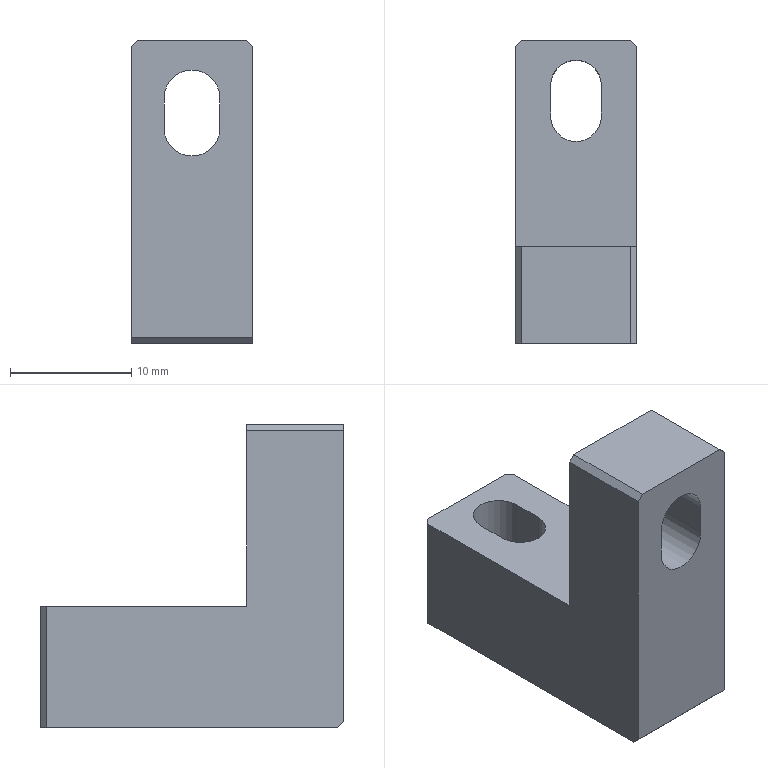Part | SolidWorks | features ICE 3, Chamfer 1, Extrusion 1, MoveFace 1 | 1 solid | 22 faces | box 10 x 25 x 25 mm | volume 3226 mm3 | plane 17 | cylinder 5 | commonest cylinder face diameters 4.6 x3 4.2 x2
STEP:
#1=CARTESIAN_POINT('',(5.,-5.,22.55));
#2=VERTEX_POINT('',#1);
#3=CARTESIAN_POINT('',(7.3,-5.,20.25));
#4=VERTEX_POINT('',#3);
#5=CARTESIAN_POINT('',(5.,-5.,20.25));
#6=DIRECTION('',(0.,1.,0.));
#7=DIRECTION('',(0.,0.,1.));
#8=AXIS2_PLACEMENT_3D('',#5,#6,#7);
#9=CIRCLE('',#8,2.3);
#10=EDGE_CURVE('',#2,#4,#9,.T.);
#11=ORIENTED_EDGE('',*,*,#10,.F.);
#12=CARTESIAN_POINT('',(5.,3.,22.55));
#13=VERTEX_POINT('',#12);
#14=CARTESIAN_POINT('',(5.,-2.,22.55));
#15=DIRECTION('',(0.,1.,0.));
#16=VECTOR('',#15,1000.);
#17=LINE('',#14,#16);
#18=EDGE_CURVE('',#2,#13,#17,.T.);
#19=ORIENTED_EDGE('',*,*,#18,.T.);
#20=CARTESIAN_POINT('',(7.3,3.,20.25));
#21=VERTEX_POINT('',#20);
#22=CARTESIAN_POINT('',(5.,3.,20.25));
#23=DIRECTION('',(0.,1.,0.));
#24=DIRECTION('',(0.,0.,1.));
#25=AXIS2_PLACEMENT_3D('',#22,#23,#24);
#26=CIRCLE('',#25,2.3);
#27=EDGE_CURVE('',#13,#21,#26,.T.);
#28=ORIENTED_EDGE('',*,*,#27,.T.);
#29=CARTESIAN_POINT('',(7.3,-2.,20.25));
#30=DIRECTION('',(0.,1.,0.));
#31=VECTOR('',#30,1000.);
#32=LINE('',#29,#31);
#33=EDGE_CURVE('',#4,#21,#32,.T.);
#34=ORIENTED_EDGE('',*,*,#33,.F.);
#35=EDGE_LOOP('',(#11,#19,#28,#34));
#36=FACE_OUTER_BOUND('',#35,.T.);
#37=CARTESIAN_POINT('',(5.,-2.,20.25));
#38=DIRECTION('',(0.,1.,0.));
#39=DIRECTION('',(0.,0.,1.));
#40=AXIS2_PLACEMENT_3D('',#37,#38,#39);
#41=CYLINDRICAL_SURFACE('',#40,2.3);
#42=ADVANCED_FACE('',(#36),#41,.F.);
#43=CARTESIAN_POINT('',(2.9,16.25,10.));
#44=VERTEX_POINT('',#43);
#45=CARTESIAN_POINT('',(2.9,13.75,10.));
#46=VERTEX_POINT('',#45);
#47=CARTESIAN_POINT('',(2.9,16.25,10.));
#48=DIRECTION('',(0.,-1.,0.));
#49=VECTOR('',#48,1000.);
#50=LINE('',#47,#49);
#51=EDGE_CURVE('',#44,#46,#50,.T.);
#52=ORIENTED_EDGE('',*,*,#51,.F.);
#53=CARTESIAN_POINT('',(7.1,16.25,10.));
#54=VERTEX_POINT('',#53);
#55=CARTESIAN_POINT('',(5.,16.25,10.));
#56=DIRECTION('',(0.,0.,1.));
#57=DIRECTION('',(1.,0.,0.));
#58=AXIS2_PLACEMENT_3D('',#55,#56,#57);
#59=CIRCLE('',#58,2.1);
#60=EDGE_CURVE('',#54,#44,#59,.T.);
#61=ORIENTED_EDGE('',*,*,#60,.F.);
#62=CARTESIAN_POINT('',(7.1,13.75,10.));
#63=VERTEX_POINT('',#62);
#64=CARTESIAN_POINT('',(7.1,16.25,10.));
#65=DIRECTION('',(0.,1.,0.));
#66=VECTOR('',#65,1000.);
#67=LINE('',#64,#66);
#68=EDGE_CURVE('',#63,#54,#67,.T.);
#69=ORIENTED_EDGE('',*,*,#68,.F.);
#70=CARTESIAN_POINT('',(5.,13.75,10.));
#71=DIRECTION('',(0.,0.,1.));
#72=DIRECTION('',(1.,0.,0.));
#73=AXIS2_PLACEMENT_3D('',#70,#71,#72);
#74=CIRCLE('',#73,2.1);
#75=EDGE_CURVE('',#46,#63,#74,.T.);
#76=ORIENTED_EDGE('',*,*,#75,.F.);
#77=EDGE_LOOP('',(#52,#61,#69,#76));
#78=FACE_BOUND('',#77,.T.);
#79=CARTESIAN_POINT('',(10.,3.,10.));
#80=VERTEX_POINT('',#79);
#81=CARTESIAN_POINT('',(10.,19.5,10.));
#82=VERTEX_POINT('',#81);
#83=CARTESIAN_POINT('',(10.,0.,10.));
#84=DIRECTION('',(0.,1.,0.));
#85=VECTOR('',#84,1000.);
#86=LINE('',#83,#85);
#87=EDGE_CURVE('',#80,#82,#86,.T.);
#88=ORIENTED_EDGE('',*,*,#87,.T.);
#89=CARTESIAN_POINT('',(9.5,20.,10.));
#90=VERTEX_POINT('',#89);
#91=CARTESIAN_POINT('',(9.5,20.,10.));
#92=DIRECTION('',(-0.7071,0.7071,0.));
#93=VECTOR('',#92,1000.);
#94=LINE('',#91,#93);
#95=EDGE_CURVE('',#82,#90,#94,.T.);
#96=ORIENTED_EDGE('',*,*,#95,.T.);
#97=CARTESIAN_POINT('',(0.5,20.,10.));
#98=VERTEX_POINT('',#97);
#99=CARTESIAN_POINT('',(0.,20.,10.));
#100=DIRECTION('',(-1.,0.,0.));
#101=VECTOR('',#100,1000.);
#102=LINE('',#99,#101);
#103=EDGE_CURVE('',#90,#98,#102,.T.);
#104=ORIENTED_EDGE('',*,*,#103,.T.);
#105=CARTESIAN_POINT('',(0.,19.5,10.));
#106=VERTEX_POINT('',#105);
#107=CARTESIAN_POINT('',(0.,19.5,10.));
#108=DIRECTION('',(-0.7071,-0.7071,0.));
#109=VECTOR('',#108,1000.);
#110=LINE('',#107,#109);
#111=EDGE_CURVE('',#98,#106,#110,.T.);
#112=ORIENTED_EDGE('',*,*,#111,.T.);
#113=CARTESIAN_POINT('',(0.,3.,10.));
#114=VERTEX_POINT('',#113);
#115=CARTESIAN_POINT('',(0.,0.,10.));
#116=DIRECTION('',(0.,-1.,0.));
#117=VECTOR('',#116,1000.);
#118=LINE('',#115,#117);
#119=EDGE_CURVE('',#106,#114,#118,.T.);
#120=ORIENTED_EDGE('',*,*,#119,.T.);
#121=CARTESIAN_POINT('',(0.,3.,10.));
#122=DIRECTION('',(-1.,0.,0.));
#123=VECTOR('',#122,1000.);
#124=LINE('',#121,#123);
#125=EDGE_CURVE('',#80,#114,#124,.T.);
#126=ORIENTED_EDGE('',*,*,#125,.F.);
#127=EDGE_LOOP('',(#88,#96,#104,#112,#120,#126));
#128=FACE_OUTER_BOUND('',#127,.T.);
#129=CARTESIAN_POINT('',(0.,0.,10.));
#130=DIRECTION('',(0.,0.,-1.));
#131=DIRECTION('',(-1.,0.,0.));
#132=AXIS2_PLACEMENT_3D('',#129,#130,#131);
#133=PLANE('',#132);
#134=ADVANCED_FACE('',(#78,#128),#133,.F.);
#135=CARTESIAN_POINT('',(0.,19.5,0.));
#136=VERTEX_POINT('',#135);
#137=CARTESIAN_POINT('',(0.,-4.5,0.));
#138=VERTEX_POINT('',#137);
#139=CARTESIAN_POINT('',(0.,0.,0.));
#140=DIRECTION('',(0.,-1.,0.));
#141=VECTOR('',#140,1000.);
#142=LINE('',#139,#141);
#143=EDGE_CURVE('',#136,#138,#142,.T.);
#144=ORIENTED_EDGE('',*,*,#143,.T.);
#145=CARTESIAN_POINT('',(0.,-5.,0.5));
#146=VERTEX_POINT('',#145);
#147=CARTESIAN_POINT('',(0.,-5.,0.5));
#148=DIRECTION('',(0.,-0.7071,0.7071));
#149=VECTOR('',#148,1000.);
#150=LINE('',#147,#149);
#151=EDGE_CURVE('',#138,#146,#150,.T.);
#152=ORIENTED_EDGE('',*,*,#151,.T.);
#153=CARTESIAN_POINT('',(0.,-5.,24.5));
#154=VERTEX_POINT('',#153);
#155=CARTESIAN_POINT('',(0.,-5.,10.));
#156=DIRECTION('',(0.,0.,-1.));
#157=VECTOR('',#156,1000.);
#158=LINE('',#155,#157);
#159=EDGE_CURVE('',#154,#146,#158,.T.);
#160=ORIENTED_EDGE('',*,*,#159,.F.);
#161=CARTESIAN_POINT('',(0.,3.,24.5));
#162=VERTEX_POINT('',#161);
#163=CARTESIAN_POINT('',(0.,0.,24.5));
#164=DIRECTION('',(0.,1.,0.));
#165=VECTOR('',#164,1000.);
#166=LINE('',#163,#165);
#167=EDGE_CURVE('',#154,#162,#166,.T.);
#168=ORIENTED_EDGE('',*,*,#167,.T.);
#169=CARTESIAN_POINT('',(0.,3.,25.));
#170=DIRECTION('',(0.,0.,-1.));
#171=VECTOR('',#170,1000.);
#172=LINE('',#169,#171);
#173=EDGE_CURVE('',#162,#114,#172,.T.);
#174=ORIENTED_EDGE('',*,*,#173,.T.);
#175=ORIENTED_EDGE('',*,*,#119,.F.);
#176=CARTESIAN_POINT('',(0.,19.5,10.));
#177=DIRECTION('',(0.,0.,-1.));
#178=VECTOR('',#177,1000.);
#179=LINE('',#176,#178);
#180=EDGE_CURVE('',#106,#136,#179,.T.);
#181=ORIENTED_EDGE('',*,*,#180,.T.);
#182=EDGE_LOOP('',(#144,#152,#160,#168,#174,#175,#181));
#183=FACE_OUTER_BOUND('',#182,.T.);
#184=CARTESIAN_POINT('',(0.,0.,10.));
#185=DIRECTION('',(1.,0.,0.));
#186=DIRECTION('',(0.,1.,0.));
#187=AXIS2_PLACEMENT_3D('',#184,#185,#186);
#188=PLANE('',#187);
#189=ADVANCED_FACE('',(#183),#188,.F.);
#190=CARTESIAN_POINT('',(2.7,-5.,17.75));
#191=VERTEX_POINT('',#190);
#192=CARTESIAN_POINT('',(2.7,-5.,20.25));
#193=VERTEX_POINT('',#192);
#194=CARTESIAN_POINT('',(2.7,-5.,10.));
#195=DIRECTION('',(0.,0.,1.));
#196=VECTOR('',#195,1000.);
#197=LINE('',#194,#196);
#198=EDGE_CURVE('',#191,#193,#197,.T.);
#199=ORIENTED_EDGE('',*,*,#198,.T.);
#200=CARTESIAN_POINT('',(5.,-5.,20.25));
#201=DIRECTION('',(0.,1.,0.));
#202=DIRECTION('',(0.,0.,1.));
#203=AXIS2_PLACEMENT_3D('',#200,#201,#202);
#204=CIRCLE('',#203,2.3);
#205=EDGE_CURVE('',#193,#2,#204,.T.);
#206=ORIENTED_EDGE('',*,*,#205,.T.);
#207=ORIENTED_EDGE('',*,*,#10,.T.);
#208=CARTESIAN_POINT('',(7.3,-5.,17.75));
#209=VERTEX_POINT('',#208);
#210=CARTESIAN_POINT('',(7.3,-5.,10.));
#211=DIRECTION('',(0.,0.,-1.));
#212=VECTOR('',#211,1000.);
#213=LINE('',#210,#212);
#214=EDGE_CURVE('',#4,#209,#213,.T.);
#215=ORIENTED_EDGE('',*,*,#214,.T.);
#216=CARTESIAN_POINT('',(5.,-5.,17.75));
#217=DIRECTION('',(0.,1.,0.));
#218=DIRECTION('',(0.,0.,1.));
#219=AXIS2_PLACEMENT_3D('',#216,#217,#218);
#220=CIRCLE('',#219,2.3);
#221=EDGE_CURVE('',#209,#191,#220,.T.);
#222=ORIENTED_EDGE('',*,*,#221,.T.);
#223=EDGE_LOOP('',(#199,#206,#207,#215,#222));
#224=FACE_BOUND('',#223,.T.);
#225=ORIENTED_EDGE('',*,*,#159,.T.);
#226=CARTESIAN_POINT('',(10.,-5.,0.5));
#227=VERTEX_POINT('',#226);
#228=CARTESIAN_POINT('',(10.,-5.,0.5));
#229=DIRECTION('',(1.,0.,0.));
#230=VECTOR('',#229,1000.);
#231=LINE('',#228,#230);
#232=EDGE_CURVE('',#146,#227,#231,.T.);
#233=ORIENTED_EDGE('',*,*,#232,.T.);
#234=CARTESIAN_POINT('',(10.,-5.,24.5));
#235=VERTEX_POINT('',#234);
#236=CARTESIAN_POINT('',(10.,-5.,10.));
#237=DIRECTION('',(0.,0.,-1.));
#238=VECTOR('',#237,1000.);
#239=LINE('',#236,#238);
#240=EDGE_CURVE('',#235,#227,#239,.T.);
#241=ORIENTED_EDGE('',*,*,#240,.F.);
#242=CARTESIAN_POINT('',(9.5,-5.,25.));
#243=VERTEX_POINT('',#242);
#244=CARTESIAN_POINT('',(9.5,-5.,25.));
#245=DIRECTION('',(-0.7071,0.,0.7071));
#246=VECTOR('',#245,1000.);
#247=LINE('',#244,#246);
#248=EDGE_CURVE('',#235,#243,#247,.T.);
#249=ORIENTED_EDGE('',*,*,#248,.T.);
#250=CARTESIAN_POINT('',(0.5,-5.,25.));
#251=VERTEX_POINT('',#250);
#252=CARTESIAN_POINT('',(0.,-5.,25.));
#253=DIRECTION('',(1.,0.,0.));
#254=VECTOR('',#253,1000.);
#255=LINE('',#252,#254);
#256=EDGE_CURVE('',#251,#243,#255,.T.);
#257=ORIENTED_EDGE('',*,*,#256,.F.);
#258=CARTESIAN_POINT('',(0.5,-5.,25.));
#259=DIRECTION('',(-0.7071,0.,-0.7071));
#260=VECTOR('',#259,1000.);
#261=LINE('',#258,#260);
#262=EDGE_CURVE('',#251,#154,#261,.T.);
#263=ORIENTED_EDGE('',*,*,#262,.T.);
#264=EDGE_LOOP('',(#225,#233,#241,#249,#257,#263));
#265=FACE_OUTER_BOUND('',#264,.T.);
#266=CARTESIAN_POINT('',(0.,-5.,10.));
#267=DIRECTION('',(0.,1.,0.));
#268=DIRECTION('',(0.,0.,1.));
#269=AXIS2_PLACEMENT_3D('',#266,#267,#268);
#270=PLANE('',#269);
#271=ADVANCED_FACE('',(#224,#265),#270,.F.);
#272=ORIENTED_EDGE('',*,*,#240,.T.);
#273=CARTESIAN_POINT('',(10.,-4.5,0.));
#274=VERTEX_POINT('',#273);
#275=CARTESIAN_POINT('',(10.,-5.,0.5));
#276=DIRECTION('',(0.,0.7071,-0.7071));
#277=VECTOR('',#276,1000.);
#278=LINE('',#275,#277);
#279=EDGE_CURVE('',#227,#274,#278,.T.);
#280=ORIENTED_EDGE('',*,*,#279,.T.);
#281=CARTESIAN_POINT('',(10.,19.5,0.));
#282=VERTEX_POINT('',#281);
#283=CARTESIAN_POINT('',(10.,0.,0.));
#284=DIRECTION('',(0.,1.,0.));
#285=VECTOR('',#284,1000.);
#286=LINE('',#283,#285);
#287=EDGE_CURVE('',#274,#282,#286,.T.);
#288=ORIENTED_EDGE('',*,*,#287,.T.);
#289=CARTESIAN_POINT('',(10.,19.5,10.));
#290=DIRECTION('',(0.,0.,1.));
#291=VECTOR('',#290,1000.);
#292=LINE('',#289,#291);
#293=EDGE_CURVE('',#282,#82,#292,.T.);
#294=ORIENTED_EDGE('',*,*,#293,.T.);
#295=ORIENTED_EDGE('',*,*,#87,.F.);
#296=CARTESIAN_POINT('',(10.,3.,24.5));
#297=VERTEX_POINT('',#296);
#298=CARTESIAN_POINT('',(10.,3.,25.));
#299=DIRECTION('',(0.,0.,-1.));
#300=VECTOR('',#299,1000.);
#301=LINE('',#298,#300);
#302=EDGE_CURVE('',#297,#80,#301,.T.);
#303=ORIENTED_EDGE('',*,*,#302,.F.);
#304=CARTESIAN_POINT('',(10.,0.,24.5));
#305=DIRECTION('',(0.,-1.,0.));
#306=VECTOR('',#305,1000.);
#307=LINE('',#304,#306);
#308=EDGE_CURVE('',#297,#235,#307,.T.);
#309=ORIENTED_EDGE('',*,*,#308,.T.);
#310=EDGE_LOOP('',(#272,#280,#288,#294,#295,#303,#309));
#311=FACE_OUTER_BOUND('',#310,.T.);
#312=CARTESIAN_POINT('',(10.,0.,10.));
#313=DIRECTION('',(-1.,0.,0.));
#314=DIRECTION('',(0.,-1.,0.));
#315=AXIS2_PLACEMENT_3D('',#312,#313,#314);
#316=PLANE('',#315);
#317=ADVANCED_FACE('',(#311),#316,.F.);
#318=ORIENTED_EDGE('',*,*,#103,.F.);
#319=CARTESIAN_POINT('',(9.5,20.,0.));
#320=VERTEX_POINT('',#319);
#321=CARTESIAN_POINT('',(9.5,20.,10.));
#322=DIRECTION('',(0.,0.,-1.));
#323=VECTOR('',#322,1000.);
#324=LINE('',#321,#323);
#325=EDGE_CURVE('',#90,#320,#324,.T.);
#326=ORIENTED_EDGE('',*,*,#325,.T.);
#327=CARTESIAN_POINT('',(0.5,20.,0.));
#328=VERTEX_POINT('',#327);
#329=CARTESIAN_POINT('',(0.,20.,0.));
#330=DIRECTION('',(-1.,0.,0.));
#331=VECTOR('',#330,1000.);
#332=LINE('',#329,#331);
#333=EDGE_CURVE('',#320,#328,#332,.T.);
#334=ORIENTED_EDGE('',*,*,#333,.T.);
#335=CARTESIAN_POINT('',(0.5,20.,10.));
#336=DIRECTION('',(0.,0.,1.));
#337=VECTOR('',#336,1000.);
#338=LINE('',#335,#337);
#339=EDGE_CURVE('',#328,#98,#338,.T.);
#340=ORIENTED_EDGE('',*,*,#339,.T.);
#341=EDGE_LOOP('',(#318,#326,#334,#340));
#342=FACE_OUTER_BOUND('',#341,.T.);
#343=CARTESIAN_POINT('',(0.,20.,10.));
#344=DIRECTION('',(0.,-1.,0.));
#345=DIRECTION('',(0.,0.,-1.));
#346=AXIS2_PLACEMENT_3D('',#343,#344,#345);
#347=PLANE('',#346);
#348=ADVANCED_FACE('',(#342),#347,.F.);
#349=CARTESIAN_POINT('',(7.1,16.25,0.));
#350=VERTEX_POINT('',#349);
#351=CARTESIAN_POINT('',(2.9,16.25,0.));
#352=VERTEX_POINT('',#351);
#353=CARTESIAN_POINT('',(5.,16.25,0.));
#354=DIRECTION('',(0.,0.,1.));
#355=DIRECTION('',(1.,0.,0.));
#356=AXIS2_PLACEMENT_3D('',#353,#354,#355);
#357=CIRCLE('',#356,2.1);
#358=EDGE_CURVE('',#350,#352,#357,.T.);
#359=ORIENTED_EDGE('',*,*,#358,.T.);
#360=CARTESIAN_POINT('',(2.9,13.75,0.));
#361=VERTEX_POINT('',#360);
#362=CARTESIAN_POINT('',(2.9,16.25,0.));
#363=DIRECTION('',(0.,-1.,0.));
#364=VECTOR('',#363,1000.);
#365=LINE('',#362,#364);
#366=EDGE_CURVE('',#352,#361,#365,.T.);
#367=ORIENTED_EDGE('',*,*,#366,.T.);
#368=CARTESIAN_POINT('',(7.1,13.75,0.));
#369=VERTEX_POINT('',#368);
#370=CARTESIAN_POINT('',(5.,13.75,0.));
#371=DIRECTION('',(0.,0.,1.));
#372=DIRECTION('',(1.,0.,0.));
#373=AXIS2_PLACEMENT_3D('',#370,#371,#372);
#374=CIRCLE('',#373,2.1);
#375=EDGE_CURVE('',#361,#369,#374,.T.);
#376=ORIENTED_EDGE('',*,*,#375,.T.);
#377=CARTESIAN_POINT('',(7.1,16.25,0.));
#378=DIRECTION('',(0.,1.,0.));
#379=VECTOR('',#378,1000.);
#380=LINE('',#377,#379);
#381=EDGE_CURVE('',#369,#350,#380,.T.);
#382=ORIENTED_EDGE('',*,*,#381,.T.);
#383=EDGE_LOOP('',(#359,#367,#376,#382));
#384=FACE_BOUND('',#383,.T.);
#385=ORIENTED_EDGE('',*,*,#287,.F.);
#386=CARTESIAN_POINT('',(0.,-4.5,0.));
#387=DIRECTION('',(-1.,0.,0.));
#388=VECTOR('',#387,1000.);
#389=LINE('',#386,#388);
#390=EDGE_CURVE('',#274,#138,#389,.T.);
#391=ORIENTED_EDGE('',*,*,#390,.T.);
#392=ORIENTED_EDGE('',*,*,#143,.F.);
#393=CARTESIAN_POINT('',(-9.75,9.75,0.));
#394=DIRECTION('',(0.7071,0.7071,0.));
#395=VECTOR('',#394,1000.);
#396=LINE('',#393,#395);
#397=EDGE_CURVE('',#136,#328,#396,.T.);
#398=ORIENTED_EDGE('',*,*,#397,.T.);
#399=ORIENTED_EDGE('',*,*,#333,.F.);
#400=CARTESIAN_POINT('',(14.75,14.75,0.));
#401=DIRECTION('',(0.7071,-0.7071,0.));
#402=VECTOR('',#401,1000.);
#403=LINE('',#400,#402);
#404=EDGE_CURVE('',#320,#282,#403,.T.);
#405=ORIENTED_EDGE('',*,*,#404,.T.);
#406=EDGE_LOOP('',(#385,#391,#392,#398,#399,#405));
#407=FACE_OUTER_BOUND('',#406,.T.);
#408=CARTESIAN_POINT('',(0.,0.,0.));
#409=DIRECTION('',(0.,0.,-1.));
#410=DIRECTION('',(-1.,0.,0.));
#411=AXIS2_PLACEMENT_3D('',#408,#409,#410);
#412=PLANE('',#411);
#413=ADVANCED_FACE('',(#384,#407),#412,.T.);
#414=CARTESIAN_POINT('',(7.3,3.,17.75));
#415=VERTEX_POINT('',#414);
#416=CARTESIAN_POINT('',(7.3,3.,20.25));
#417=DIRECTION('',(0.,0.,-1.));
#418=VECTOR('',#417,1000.);
#419=LINE('',#416,#418);
#420=EDGE_CURVE('',#21,#415,#419,.T.);
#421=ORIENTED_EDGE('',*,*,#420,.F.);
#422=ORIENTED_EDGE('',*,*,#27,.F.);
#423=CARTESIAN_POINT('',(2.7,3.,20.25));
#424=VERTEX_POINT('',#423);
#425=CARTESIAN_POINT('',(5.,3.,20.25));
#426=DIRECTION('',(0.,1.,0.));
#427=DIRECTION('',(0.,0.,1.));
#428=AXIS2_PLACEMENT_3D('',#425,#426,#427);
#429=CIRCLE('',#428,2.3);
#430=EDGE_CURVE('',#424,#13,#429,.T.);
#431=ORIENTED_EDGE('',*,*,#430,.F.);
#432=CARTESIAN_POINT('',(2.7,3.,17.75));
#433=VERTEX_POINT('',#432);
#434=CARTESIAN_POINT('',(2.7,3.,20.25));
#435=DIRECTION('',(0.,0.,1.));
#436=VECTOR('',#435,1000.);
#437=LINE('',#434,#436);
#438=EDGE_CURVE('',#433,#424,#437,.T.);
#439=ORIENTED_EDGE('',*,*,#438,.F.);
#440=CARTESIAN_POINT('',(5.,3.,17.75));
#441=DIRECTION('',(0.,1.,0.));
#442=DIRECTION('',(0.,0.,1.));
#443=AXIS2_PLACEMENT_3D('',#440,#441,#442);
#444=CIRCLE('',#443,2.3);
#445=EDGE_CURVE('',#415,#433,#444,.T.);
#446=ORIENTED_EDGE('',*,*,#445,.F.);
#447=EDGE_LOOP('',(#421,#422,#431,#439,#446));
#448=FACE_BOUND('',#447,.T.);
#449=CARTESIAN_POINT('',(9.5,3.,25.));
#450=VERTEX_POINT('',#449);
#451=CARTESIAN_POINT('',(0.5,3.,25.));
#452=VERTEX_POINT('',#451);
#453=CARTESIAN_POINT('',(0.,3.,25.));
#454=DIRECTION('',(-1.,0.,0.));
#455=VECTOR('',#454,1000.);
#456=LINE('',#453,#455);
#457=EDGE_CURVE('',#450,#452,#456,.T.);
#458=ORIENTED_EDGE('',*,*,#457,.F.);
#459=CARTESIAN_POINT('',(9.5,3.,25.));
#460=DIRECTION('',(0.7071,0.,-0.7071));
#461=VECTOR('',#460,1000.);
#462=LINE('',#459,#461);
#463=EDGE_CURVE('',#450,#297,#462,.T.);
#464=ORIENTED_EDGE('',*,*,#463,.T.);
#465=ORIENTED_EDGE('',*,*,#302,.T.);
#466=ORIENTED_EDGE('',*,*,#125,.T.);
#467=ORIENTED_EDGE('',*,*,#173,.F.);
#468=CARTESIAN_POINT('',(0.5,3.,25.));
#469=DIRECTION('',(0.7071,0.,0.7071));
#470=VECTOR('',#469,1000.);
#471=LINE('',#468,#470);
#472=EDGE_CURVE('',#162,#452,#471,.T.);
#473=ORIENTED_EDGE('',*,*,#472,.T.);
#474=EDGE_LOOP('',(#458,#464,#465,#466,#467,#473));
#475=FACE_OUTER_BOUND('',#474,.T.);
#476=CARTESIAN_POINT('',(0.,3.,25.));
#477=DIRECTION('',(0.,-1.,0.));
#478=DIRECTION('',(0.,0.,-1.));
#479=AXIS2_PLACEMENT_3D('',#476,#477,#478);
#480=PLANE('',#479);
#481=ADVANCED_FACE('',(#448,#475),#480,.F.);
#482=ORIENTED_EDGE('',*,*,#256,.T.);
#483=CARTESIAN_POINT('',(9.5,0.,25.));
#484=DIRECTION('',(0.,1.,0.));
#485=VECTOR('',#484,1000.);
#486=LINE('',#483,#485);
#487=EDGE_CURVE('',#243,#450,#486,.T.);
#488=ORIENTED_EDGE('',*,*,#487,.T.);
#489=ORIENTED_EDGE('',*,*,#457,.T.);
#490=CARTESIAN_POINT('',(0.5,0.,25.));
#491=DIRECTION('',(0.,-1.,0.));
#492=VECTOR('',#491,1000.);
#493=LINE('',#490,#492);
#494=EDGE_CURVE('',#452,#251,#493,.T.);
#495=ORIENTED_EDGE('',*,*,#494,.T.);
#496=EDGE_LOOP('',(#482,#488,#489,#495));
#497=FACE_OUTER_BOUND('',#496,.T.);
#498=CARTESIAN_POINT('',(0.,0.,25.));
#499=DIRECTION('',(0.,0.,-1.));
#500=DIRECTION('',(-1.,0.,0.));
#501=AXIS2_PLACEMENT_3D('',#498,#499,#500);
#502=PLANE('',#501);
#503=ADVANCED_FACE('',(#497),#502,.F.);
#504=ORIENTED_EDGE('',*,*,#60,.T.);
#505=CARTESIAN_POINT('',(2.9,16.25,0.));
#506=DIRECTION('',(0.,0.,1.));
#507=VECTOR('',#506,1000.);
#508=LINE('',#505,#507);
#509=EDGE_CURVE('',#352,#44,#508,.T.);
#510=ORIENTED_EDGE('',*,*,#509,.F.);
#511=ORIENTED_EDGE('',*,*,#358,.F.);
#512=CARTESIAN_POINT('',(7.1,16.25,0.));
#513=DIRECTION('',(0.,0.,1.));
#514=VECTOR('',#513,1000.);
#515=LINE('',#512,#514);
#516=EDGE_CURVE('',#350,#54,#515,.T.);
#517=ORIENTED_EDGE('',*,*,#516,.T.);
#518=EDGE_LOOP('',(#504,#510,#511,#517));
#519=FACE_OUTER_BOUND('',#518,.T.);
#520=CARTESIAN_POINT('',(5.,16.25,0.));
#521=DIRECTION('',(0.,0.,1.));
#522=DIRECTION('',(1.,0.,0.));
#523=AXIS2_PLACEMENT_3D('',#520,#521,#522);
#524=CYLINDRICAL_SURFACE('',#523,2.1);
#525=ADVANCED_FACE('',(#519),#524,.F.);
#526=ORIENTED_EDGE('',*,*,#68,.T.);
#527=ORIENTED_EDGE('',*,*,#516,.F.);
#528=ORIENTED_EDGE('',*,*,#381,.F.);
#529=CARTESIAN_POINT('',(7.1,13.75,0.));
#530=DIRECTION('',(0.,0.,1.));
#531=VECTOR('',#530,1000.);
#532=LINE('',#529,#531);
#533=EDGE_CURVE('',#369,#63,#532,.T.);
#534=ORIENTED_EDGE('',*,*,#533,.T.);
#535=EDGE_LOOP('',(#526,#527,#528,#534));
#536=FACE_OUTER_BOUND('',#535,.T.);
#537=CARTESIAN_POINT('',(7.1,16.25,0.));
#538=DIRECTION('',(1.,0.,0.));
#539=DIRECTION('',(0.,1.,0.));
#540=AXIS2_PLACEMENT_3D('',#537,#538,#539);
#541=PLANE('',#540);
#542=ADVANCED_FACE('',(#536),#541,.F.);
#543=ORIENTED_EDGE('',*,*,#75,.T.);
#544=ORIENTED_EDGE('',*,*,#533,.F.);
#545=ORIENTED_EDGE('',*,*,#375,.F.);
#546=CARTESIAN_POINT('',(2.9,13.75,0.));
#547=DIRECTION('',(0.,0.,1.));
#548=VECTOR('',#547,1000.);
#549=LINE('',#546,#548);
#550=EDGE_CURVE('',#361,#46,#549,.T.);
#551=ORIENTED_EDGE('',*,*,#550,.T.);
#552=EDGE_LOOP('',(#543,#544,#545,#551));
#553=FACE_OUTER_BOUND('',#552,.T.);
#554=CARTESIAN_POINT('',(5.,13.75,0.));
#555=DIRECTION('',(0.,0.,1.));
#556=DIRECTION('',(1.,0.,0.));
#557=AXIS2_PLACEMENT_3D('',#554,#555,#556);
#558=CYLINDRICAL_SURFACE('',#557,2.1);
#559=ADVANCED_FACE('',(#553),#558,.F.);
#560=ORIENTED_EDGE('',*,*,#51,.T.);
#561=ORIENTED_EDGE('',*,*,#550,.F.);
#562=ORIENTED_EDGE('',*,*,#366,.F.);
#563=ORIENTED_EDGE('',*,*,#509,.T.);
#564=EDGE_LOOP('',(#560,#561,#562,#563));
#565=FACE_OUTER_BOUND('',#564,.T.);
#566=CARTESIAN_POINT('',(2.9,16.25,0.));
#567=DIRECTION('',(-1.,0.,0.));
#568=DIRECTION('',(0.,-1.,0.));
#569=AXIS2_PLACEMENT_3D('',#566,#567,#568);
#570=PLANE('',#569);
#571=ADVANCED_FACE('',(#565),#570,.F.);
#572=ORIENTED_EDGE('',*,*,#18,.F.);
#573=ORIENTED_EDGE('',*,*,#205,.F.);
#574=CARTESIAN_POINT('',(2.7,-2.,20.25));
#575=DIRECTION('',(0.,1.,0.));
#576=VECTOR('',#575,1000.);
#577=LINE('',#574,#576);
#578=EDGE_CURVE('',#193,#424,#577,.T.);
#579=ORIENTED_EDGE('',*,*,#578,.T.);
#580=ORIENTED_EDGE('',*,*,#430,.T.);
#581=EDGE_LOOP('',(#572,#573,#579,#580));
#582=FACE_OUTER_BOUND('',#581,.T.);
#583=CARTESIAN_POINT('',(5.,-2.,20.25));
#584=DIRECTION('',(0.,1.,0.));
#585=DIRECTION('',(0.,0.,1.));
#586=AXIS2_PLACEMENT_3D('',#583,#584,#585);
#587=CYLINDRICAL_SURFACE('',#586,2.3);
#588=ADVANCED_FACE('',(#582),#587,.F.);
#589=CARTESIAN_POINT('',(2.7,-2.,17.75));
#590=DIRECTION('',(0.,1.,0.));
#591=VECTOR('',#590,1000.);
#592=LINE('',#589,#591);
#593=EDGE_CURVE('',#191,#433,#592,.T.);
#594=ORIENTED_EDGE('',*,*,#593,.T.);
#595=ORIENTED_EDGE('',*,*,#438,.T.);
#596=ORIENTED_EDGE('',*,*,#578,.F.);
#597=ORIENTED_EDGE('',*,*,#198,.F.);
#598=EDGE_LOOP('',(#594,#595,#596,#597));
#599=FACE_OUTER_BOUND('',#598,.T.);
#600=CARTESIAN_POINT('',(2.7,-2.,20.25));
#601=DIRECTION('',(-1.,0.,0.));
#602=DIRECTION('',(0.,0.,1.));
#603=AXIS2_PLACEMENT_3D('',#600,#601,#602);
#604=PLANE('',#603);
#605=ADVANCED_FACE('',(#599),#604,.F.);
#606=CARTESIAN_POINT('',(7.3,-2.,17.75));
#607=DIRECTION('',(0.,1.,0.));
#608=VECTOR('',#607,1000.);
#609=LINE('',#606,#608);
#610=EDGE_CURVE('',#209,#415,#609,.T.);
#611=ORIENTED_EDGE('',*,*,#610,.T.);
#612=ORIENTED_EDGE('',*,*,#445,.T.);
#613=ORIENTED_EDGE('',*,*,#593,.F.);
#614=ORIENTED_EDGE('',*,*,#221,.F.);
#615=EDGE_LOOP('',(#611,#612,#613,#614));
#616=FACE_OUTER_BOUND('',#615,.T.);
#617=CARTESIAN_POINT('',(5.,-2.,17.75));
#618=DIRECTION('',(0.,1.,0.));
#619=DIRECTION('',(0.,0.,1.));
#620=AXIS2_PLACEMENT_3D('',#617,#618,#619);
#621=CYLINDRICAL_SURFACE('',#620,2.3);
#622=ADVANCED_FACE('',(#616),#621,.F.);
#623=ORIENTED_EDGE('',*,*,#33,.T.);
#624=ORIENTED_EDGE('',*,*,#420,.T.);
#625=ORIENTED_EDGE('',*,*,#610,.F.);
#626=ORIENTED_EDGE('',*,*,#214,.F.);
#627=EDGE_LOOP('',(#623,#624,#625,#626));
#628=FACE_OUTER_BOUND('',#627,.T.);
#629=CARTESIAN_POINT('',(7.3,-2.,20.25));
#630=DIRECTION('',(1.,0.,0.));
#631=DIRECTION('',(0.,0.,-1.));
#632=AXIS2_PLACEMENT_3D('',#629,#630,#631);
#633=PLANE('',#632);
#634=ADVANCED_FACE('',(#628),#633,.F.);
#635=ORIENTED_EDGE('',*,*,#151,.F.);
#636=ORIENTED_EDGE('',*,*,#390,.F.);
#637=ORIENTED_EDGE('',*,*,#279,.F.);
#638=ORIENTED_EDGE('',*,*,#232,.F.);
#639=EDGE_LOOP('',(#635,#636,#637,#638));
#640=FACE_OUTER_BOUND('',#639,.T.);
#641=CARTESIAN_POINT('',(0.,-5.,0.5));
#642=DIRECTION('',(0.,-0.7071,-0.7071));
#643=DIRECTION('',(-1.,0.,0.));
#644=AXIS2_PLACEMENT_3D('',#641,#642,#643);
#645=PLANE('',#644);
#646=ADVANCED_FACE('',(#640),#645,.T.);
#647=ORIENTED_EDGE('',*,*,#248,.F.);
#648=ORIENTED_EDGE('',*,*,#308,.F.);
#649=ORIENTED_EDGE('',*,*,#463,.F.);
#650=ORIENTED_EDGE('',*,*,#487,.F.);
#651=EDGE_LOOP('',(#647,#648,#649,#650));
#652=FACE_OUTER_BOUND('',#651,.T.);
#653=CARTESIAN_POINT('',(9.5,0.,25.));
#654=DIRECTION('',(-0.7071,0.,-0.7071));
#655=DIRECTION('',(0.,1.,0.));
#656=AXIS2_PLACEMENT_3D('',#653,#654,#655);
#657=PLANE('',#656);
#658=ADVANCED_FACE('',(#652),#657,.F.);
#659=ORIENTED_EDGE('',*,*,#472,.F.);
#660=ORIENTED_EDGE('',*,*,#167,.F.);
#661=ORIENTED_EDGE('',*,*,#262,.F.);
#662=ORIENTED_EDGE('',*,*,#494,.F.);
#663=EDGE_LOOP('',(#659,#660,#661,#662));
#664=FACE_OUTER_BOUND('',#663,.T.);
#665=CARTESIAN_POINT('',(0.5,0.,25.));
#666=DIRECTION('',(0.7071,0.,-0.7071));
#667=DIRECTION('',(0.,-1.,0.));
#668=AXIS2_PLACEMENT_3D('',#665,#666,#667);
#669=PLANE('',#668);
#670=ADVANCED_FACE('',(#664),#669,.F.);
#671=ORIENTED_EDGE('',*,*,#95,.F.);
#672=ORIENTED_EDGE('',*,*,#293,.F.);
#673=ORIENTED_EDGE('',*,*,#404,.F.);
#674=ORIENTED_EDGE('',*,*,#325,.F.);
#675=EDGE_LOOP('',(#671,#672,#673,#674));
#676=FACE_OUTER_BOUND('',#675,.T.);
#677=CARTESIAN_POINT('',(9.5,20.,10.));
#678=DIRECTION('',(-0.7071,-0.7071,0.));
#679=DIRECTION('',(0.,0.,-1.));
#680=AXIS2_PLACEMENT_3D('',#677,#678,#679);
#681=PLANE('',#680);
#682=ADVANCED_FACE('',(#676),#681,.F.);
#683=ORIENTED_EDGE('',*,*,#111,.F.);
#684=ORIENTED_EDGE('',*,*,#339,.F.);
#685=ORIENTED_EDGE('',*,*,#397,.F.);
#686=ORIENTED_EDGE('',*,*,#180,.F.);
#687=EDGE_LOOP('',(#683,#684,#685,#686));
#688=FACE_OUTER_BOUND('',#687,.T.);
#689=CARTESIAN_POINT('',(0.,19.5,10.));
#690=DIRECTION('',(0.7071,-0.7071,0.));
#691=DIRECTION('',(0.,0.,-1.));
#692=AXIS2_PLACEMENT_3D('',#689,#690,#691);
#693=PLANE('',#692);
#694=ADVANCED_FACE('',(#688),#693,.F.);
#695=CLOSED_SHELL('',(#42,#134,#189,#271,#317,#348,#413,#481,#503,#525,#542,#559,#571,#588,#605,#622,#634,#646,#658,#670,#682,#694));
#696=MANIFOLD_SOLID_BREP('',#695);
#697=CARTESIAN_POINT('',(0.,0.,0.));
#698=DIRECTION('',(0.,0.,1.));
#699=DIRECTION('',(1.,0.,0.));
#700=AXIS2_PLACEMENT_3D('',#697,#698,#699);
#701=(LENGTH_UNIT()NAMED_UNIT(*)SI_UNIT(.MILLI.,.METRE.));
#702=UNCERTAINTY_MEASURE_WITH_UNIT(LENGTH_MEASURE(0.00001),#701,'','');
#703=(NAMED_UNIT(*)PLANE_ANGLE_UNIT()SI_UNIT($,.RADIAN.));
#704=(NAMED_UNIT(*)SI_UNIT($,.STERADIAN.)SOLID_ANGLE_UNIT());
#705=(GEOMETRIC_REPRESENTATION_CONTEXT(3)GLOBAL_UNCERTAINTY_ASSIGNED_CONTEXT((#702))GLOBAL_UNIT_ASSIGNED_CONTEXT((#701,#703,#704))REPRESENTATION_CONTEXT('',''));
#706=ADVANCED_BREP_SHAPE_REPRESENTATION('',(#696,#700),#705);